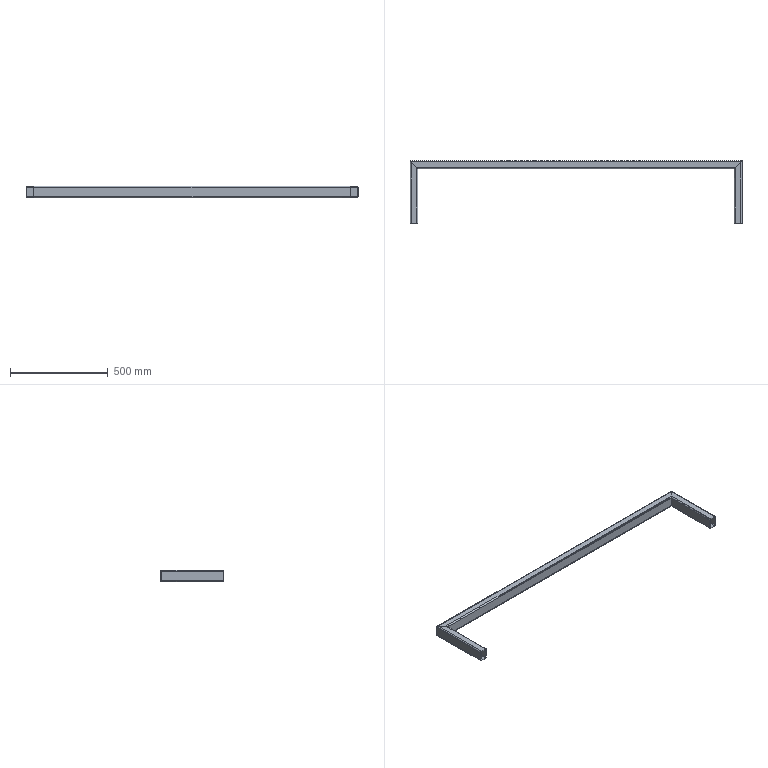Part | STEP file | Frame 1_Default<Machined> | 3 solids | 54 faces | box 1700 x 320 x 60 mm | volume 1222260 mm3 | plane 30 | cylinder 24 | commonest cylinder face diameters 6 x12 12 x12